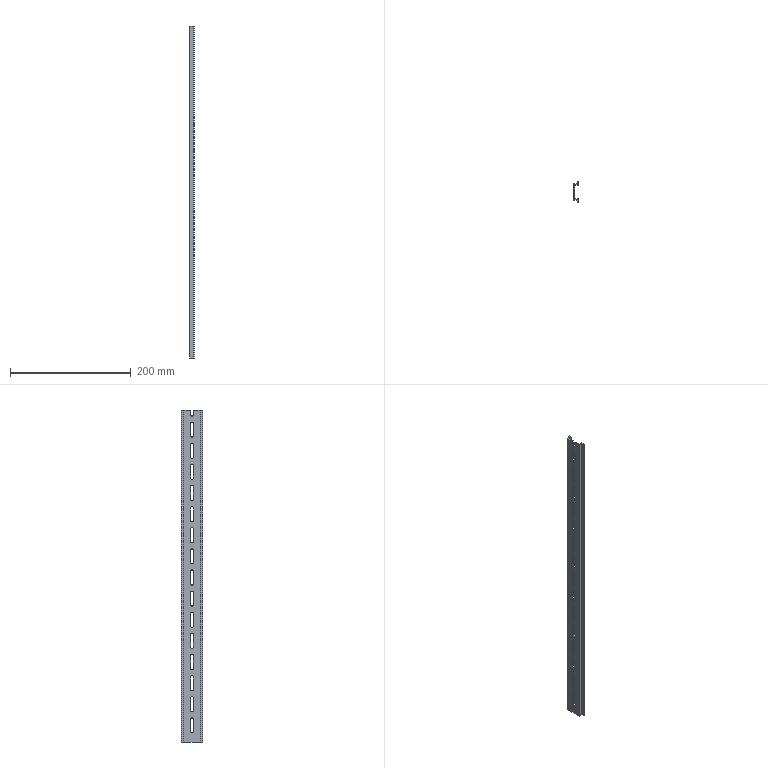Part | STEP file | [SDR-1(550L)] | 1 solid | 78 faces | box 7.5 x 35 x 550 mm | volume 36277 mm3 | plane 47 | cylinder 31 | commonest cylinder face diameters 4.5 x31